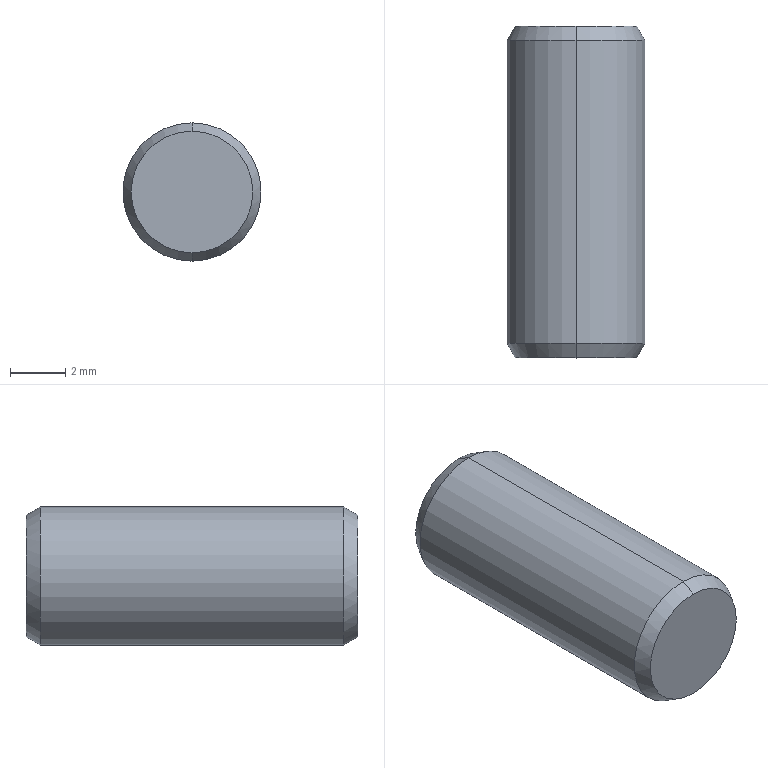Part | STEP file | 1 solid | 8 faces | box 5 x 12 x 5 mm | volume 233.269 mm3 | cone 4 | cylinder 2 | plane 2 | commonest cylinder face diameters 5 x2
STEP:
#1=CARTESIAN_POINT('',(0.,0.,0.));
#2=DIRECTION('',(0.,0.,1.));
#3=DIRECTION('',(1.,0.,0.));
#4=AXIS2_PLACEMENT_3D('',#1,#2,#3);
#5=CARTESIAN_POINT('',(0.,-12.,-2.2));
#6=VERTEX_POINT('',#5);
#7=CARTESIAN_POINT('',(0.,-12.,2.2));
#8=VERTEX_POINT('',#7);
#9=CARTESIAN_POINT('',(0.,-12.,0.));
#10=DIRECTION('',(0.,-1.,0.));
#11=DIRECTION('',(0.,0.,-1.));
#12=AXIS2_PLACEMENT_3D('',#9,#10,#11);
#13=CIRCLE('',#12,2.2);
#14=CARTESIAN_POINT('',(0.,-11.48,0.));
#15=DIRECTION('',(0.,1.,0.));
#16=DIRECTION('',(0.,0.,1.));
#17=AXIS2_PLACEMENT_3D('',#14,#15,#16);
#18=CONICAL_SURFACE('',#17,2.5,0.5236);
#19=CARTESIAN_POINT('',(3.142,-0.5196));
#20=DIRECTION('',(-1.,0.));
#21=VECTOR('',#20,1.);
#22=LINE('',#19,#21);
#23=(GEOMETRIC_REPRESENTATION_CONTEXT(2)PARAMETRIC_REPRESENTATION_CONTEXT()REPRESENTATION_CONTEXT('',''));
#24=DEFINITIONAL_REPRESENTATION('',(#22),#23);
#25=PCURVE('',#18,#24);
#26=CARTESIAN_POINT('',(-2.2,-12.,0.));
#27=DIRECTION('',(0.,1.,0.));
#28=DIRECTION('',(0.,0.,1.));
#29=AXIS2_PLACEMENT_3D('',#26,#27,#28);
#30=PLANE('',#29);
#31=CARTESIAN_POINT('',(-2.2,2.2));
#32=CARTESIAN_POINT('',(-2.2,6.011));
#33=CARTESIAN_POINT('',(1.1,4.105));
#34=CARTESIAN_POINT('',(4.4,2.2));
#35=CARTESIAN_POINT('',(1.1,0.2947));
#36=CARTESIAN_POINT('',(-2.2,-1.611));
#37=CARTESIAN_POINT('',(-2.2,2.2));
#38=(BOUNDED_CURVE()B_SPLINE_CURVE(2,(#31,#32,#33,#34,#35,#36,#37),.UNSPECIFIED.,.T.,.F.)B_SPLINE_CURVE_WITH_KNOTS((1,2,2,2,2,1),(-2.094,0.,2.094,4.189,6.283,8.378),.UNSPECIFIED.)CURVE()GEOMETRIC_REPRESENTATION_ITEM()RATIONAL_B_SPLINE_CURVE((1.,0.5,1.,0.5,1.,0.5,1.))REPRESENTATION_ITEM(''));
#39=(GEOMETRIC_REPRESENTATION_CONTEXT(2)PARAMETRIC_REPRESENTATION_CONTEXT()REPRESENTATION_CONTEXT('',''));
#40=DEFINITIONAL_REPRESENTATION('',(#38),#39);
#41=PCURVE('',#30,#40);
#42=SURFACE_CURVE('',#13,(#25,#41),.PCURVE_S1.);
#43=EDGE_CURVE('',#6,#8,#42,.T.);
#44=ORIENTED_EDGE('',*,*,#43,.F.);
#45=CARTESIAN_POINT('',(0.,-11.48,-2.5));
#46=VERTEX_POINT('',#45);
#47=CARTESIAN_POINT('',(0.,-11.48,-2.5));
#48=DIRECTION('',(0.,0.866,-0.5));
#49=VECTOR('',#48,1.);
#50=LINE('',#47,#49);
#51=CARTESIAN_POINT('',(3.142,0.));
#52=DIRECTION('',(0.,1.));
#53=VECTOR('',#52,1.);
#54=LINE('',#51,#53);
#55=(GEOMETRIC_REPRESENTATION_CONTEXT(2)PARAMETRIC_REPRESENTATION_CONTEXT()REPRESENTATION_CONTEXT('',''));
#56=DEFINITIONAL_REPRESENTATION('',(#54),#55);
#57=PCURVE('',#18,#56);
#58=CARTESIAN_POINT('',(0.,-11.48,0.));
#59=DIRECTION('',(0.,1.,0.));
#60=DIRECTION('',(0.,0.,1.));
#61=AXIS2_PLACEMENT_3D('',#58,#59,#60);
#62=CONICAL_SURFACE('',#61,2.5,0.5236);
#63=CARTESIAN_POINT('',(3.142,0.));
#64=DIRECTION('',(0.,1.));
#65=VECTOR('',#64,1.);
#66=LINE('',#63,#65);
#67=(GEOMETRIC_REPRESENTATION_CONTEXT(2)PARAMETRIC_REPRESENTATION_CONTEXT()REPRESENTATION_CONTEXT('',''));
#68=DEFINITIONAL_REPRESENTATION('',(#66),#67);
#69=PCURVE('',#62,#68);
#70=SURFACE_CURVE('',#50,(#57,#69),.PCURVE_S1.);
#71=EDGE_CURVE('',#6,#46,#70,.T.);
#72=ORIENTED_EDGE('',*,*,#71,.T.);
#73=CARTESIAN_POINT('',(0.,-11.48,2.5));
#74=VERTEX_POINT('',#73);
#75=CARTESIAN_POINT('',(0.,-11.48,0.));
#76=DIRECTION('',(0.,-1.,0.));
#77=DIRECTION('',(0.,0.,-1.));
#78=AXIS2_PLACEMENT_3D('',#75,#76,#77);
#79=CIRCLE('',#78,2.5);
#80=CARTESIAN_POINT('',(3.142,0.));
#81=DIRECTION('',(-1.,0.));
#82=VECTOR('',#81,1.);
#83=LINE('',#80,#82);
#84=(GEOMETRIC_REPRESENTATION_CONTEXT(2)PARAMETRIC_REPRESENTATION_CONTEXT()REPRESENTATION_CONTEXT('',''));
#85=DEFINITIONAL_REPRESENTATION('',(#83),#84);
#86=PCURVE('',#18,#85);
#87=CARTESIAN_POINT('',(0.,-12.,0.));
#88=DIRECTION('',(0.,-1.,0.));
#89=DIRECTION('',(0.,0.,-1.));
#90=AXIS2_PLACEMENT_3D('',#87,#88,#89);
#91=CYLINDRICAL_SURFACE('',#90,2.5);
#92=CARTESIAN_POINT('',(0.,-0.5196));
#93=DIRECTION('',(1.,0.));
#94=VECTOR('',#93,1.);
#95=LINE('',#92,#94);
#96=(GEOMETRIC_REPRESENTATION_CONTEXT(2)PARAMETRIC_REPRESENTATION_CONTEXT()REPRESENTATION_CONTEXT('',''));
#97=DEFINITIONAL_REPRESENTATION('',(#95),#96);
#98=PCURVE('',#91,#97);
#99=SURFACE_CURVE('',#79,(#86,#98),.PCURVE_S1.);
#100=EDGE_CURVE('',#46,#74,#99,.T.);
#101=ORIENTED_EDGE('',*,*,#100,.T.);
#102=CARTESIAN_POINT('',(0.,-11.48,2.5));
#103=DIRECTION('',(0.,0.866,0.5));
#104=VECTOR('',#103,1.);
#105=LINE('',#102,#104);
#106=CARTESIAN_POINT('',(0.,0.));
#107=DIRECTION('',(0.,1.));
#108=VECTOR('',#107,1.);
#109=LINE('',#106,#108);
#110=(GEOMETRIC_REPRESENTATION_CONTEXT(2)PARAMETRIC_REPRESENTATION_CONTEXT()REPRESENTATION_CONTEXT('',''));
#111=DEFINITIONAL_REPRESENTATION('',(#109),#110);
#112=PCURVE('',#18,#111);
#113=CARTESIAN_POINT('',(6.283,0.));
#114=DIRECTION('',(0.,1.));
#115=VECTOR('',#114,1.);
#116=LINE('',#113,#115);
#117=(GEOMETRIC_REPRESENTATION_CONTEXT(2)PARAMETRIC_REPRESENTATION_CONTEXT()REPRESENTATION_CONTEXT('',''));
#118=DEFINITIONAL_REPRESENTATION('',(#116),#117);
#119=PCURVE('',#62,#118);
#120=SURFACE_CURVE('',#105,(#112,#119),.PCURVE_S1.);
#121=EDGE_CURVE('',#8,#74,#120,.T.);
#122=ORIENTED_EDGE('',*,*,#121,.F.);
#123=EDGE_LOOP('',(#44,#72,#101,#122));
#124=FACE_BOUND('',#123,.T.);
#125=ADVANCED_FACE('',(#124),#18,.T.);
#126=CARTESIAN_POINT('',(0.,-0.5196,-2.5));
#127=VERTEX_POINT('',#126);
#128=CARTESIAN_POINT('',(0.,-0.5196,2.5));
#129=VERTEX_POINT('',#128);
#130=CARTESIAN_POINT('',(0.,-0.5196,0.));
#131=DIRECTION('',(0.,-1.,0.));
#132=DIRECTION('',(0.,0.,-1.));
#133=AXIS2_PLACEMENT_3D('',#130,#131,#132);
#134=CIRCLE('',#133,2.5);
#135=CARTESIAN_POINT('',(0.,-11.48));
#136=DIRECTION('',(1.,0.));
#137=VECTOR('',#136,1.);
#138=LINE('',#135,#137);
#139=(GEOMETRIC_REPRESENTATION_CONTEXT(2)PARAMETRIC_REPRESENTATION_CONTEXT()REPRESENTATION_CONTEXT('',''));
#140=DEFINITIONAL_REPRESENTATION('',(#138),#139);
#141=PCURVE('',#91,#140);
#142=CARTESIAN_POINT('',(0.,0.,0.));
#143=DIRECTION('',(0.,-1.,0.));
#144=DIRECTION('',(0.,0.,-1.));
#145=AXIS2_PLACEMENT_3D('',#142,#143,#144);
#146=CONICAL_SURFACE('',#145,2.2,0.5236);
#147=CARTESIAN_POINT('',(0.,0.5196));
#148=DIRECTION('',(1.,0.));
#149=VECTOR('',#148,1.);
#150=LINE('',#147,#149);
#151=(GEOMETRIC_REPRESENTATION_CONTEXT(2)PARAMETRIC_REPRESENTATION_CONTEXT()REPRESENTATION_CONTEXT('',''));
#152=DEFINITIONAL_REPRESENTATION('',(#150),#151);
#153=PCURVE('',#146,#152);
#154=SURFACE_CURVE('',#134,(#141,#153),.PCURVE_S1.);
#155=EDGE_CURVE('',#127,#129,#154,.T.);
#156=ORIENTED_EDGE('',*,*,#155,.T.);
#157=CARTESIAN_POINT('',(0.,-12.,2.5));
#158=DIRECTION('',(0.,-1.,0.));
#159=VECTOR('',#158,1.);
#160=LINE('',#157,#159);
#161=CARTESIAN_POINT('',(3.142,0.));
#162=DIRECTION('',(0.,1.));
#163=VECTOR('',#162,1.);
#164=LINE('',#161,#163);
#165=(GEOMETRIC_REPRESENTATION_CONTEXT(2)PARAMETRIC_REPRESENTATION_CONTEXT()REPRESENTATION_CONTEXT('',''));
#166=DEFINITIONAL_REPRESENTATION('',(#164),#165);
#167=PCURVE('',#91,#166);
#168=CARTESIAN_POINT('',(0.,-12.,0.));
#169=DIRECTION('',(0.,-1.,0.));
#170=DIRECTION('',(0.,0.,-1.));
#171=AXIS2_PLACEMENT_3D('',#168,#169,#170);
#172=CYLINDRICAL_SURFACE('',#171,2.5);
#173=CARTESIAN_POINT('',(3.142,0.));
#174=DIRECTION('',(0.,1.));
#175=VECTOR('',#174,1.);
#176=LINE('',#173,#175);
#177=(GEOMETRIC_REPRESENTATION_CONTEXT(2)PARAMETRIC_REPRESENTATION_CONTEXT()REPRESENTATION_CONTEXT('',''));
#178=DEFINITIONAL_REPRESENTATION('',(#176),#177);
#179=PCURVE('',#172,#178);
#180=SURFACE_CURVE('',#160,(#167,#179),.PCURVE_S1.);
#181=EDGE_CURVE('',#129,#74,#180,.T.);
#182=ORIENTED_EDGE('',*,*,#181,.T.);
#183=ORIENTED_EDGE('',*,*,#100,.F.);
#184=CARTESIAN_POINT('',(0.,-12.,-2.5));
#185=DIRECTION('',(0.,-1.,0.));
#186=VECTOR('',#185,1.);
#187=LINE('',#184,#186);
#188=CARTESIAN_POINT('',(0.,0.));
#189=DIRECTION('',(0.,1.));
#190=VECTOR('',#189,1.);
#191=LINE('',#188,#190);
#192=(GEOMETRIC_REPRESENTATION_CONTEXT(2)PARAMETRIC_REPRESENTATION_CONTEXT()REPRESENTATION_CONTEXT('',''));
#193=DEFINITIONAL_REPRESENTATION('',(#191),#192);
#194=PCURVE('',#91,#193);
#195=CARTESIAN_POINT('',(6.283,0.));
#196=DIRECTION('',(0.,1.));
#197=VECTOR('',#196,1.);
#198=LINE('',#195,#197);
#199=(GEOMETRIC_REPRESENTATION_CONTEXT(2)PARAMETRIC_REPRESENTATION_CONTEXT()REPRESENTATION_CONTEXT('',''));
#200=DEFINITIONAL_REPRESENTATION('',(#198),#199);
#201=PCURVE('',#172,#200);
#202=SURFACE_CURVE('',#187,(#194,#201),.PCURVE_S1.);
#203=EDGE_CURVE('',#127,#46,#202,.T.);
#204=ORIENTED_EDGE('',*,*,#203,.F.);
#205=EDGE_LOOP('',(#156,#182,#183,#204));
#206=FACE_BOUND('',#205,.T.);
#207=ADVANCED_FACE('',(#206),#91,.T.);
#208=CARTESIAN_POINT('',(0.,0.,-2.2));
#209=VERTEX_POINT('',#208);
#210=CARTESIAN_POINT('',(0.,0.,2.2));
#211=VERTEX_POINT('',#210);
#212=CARTESIAN_POINT('',(0.,0.,0.));
#213=DIRECTION('',(0.,-1.,0.));
#214=DIRECTION('',(0.,0.,-1.));
#215=AXIS2_PLACEMENT_3D('',#212,#213,#214);
#216=CIRCLE('',#215,2.2);
#217=CARTESIAN_POINT('',(0.,0.));
#218=DIRECTION('',(1.,0.));
#219=VECTOR('',#218,1.);
#220=LINE('',#217,#219);
#221=(GEOMETRIC_REPRESENTATION_CONTEXT(2)PARAMETRIC_REPRESENTATION_CONTEXT()REPRESENTATION_CONTEXT('',''));
#222=DEFINITIONAL_REPRESENTATION('',(#220),#221);
#223=PCURVE('',#146,#222);
#224=CARTESIAN_POINT('',(0.,0.,0.));
#225=DIRECTION('',(0.,-1.,0.));
#226=DIRECTION('',(0.,0.,-1.));
#227=AXIS2_PLACEMENT_3D('',#224,#225,#226);
#228=PLANE('',#227);
#229=CARTESIAN_POINT('',(0.,0.));
#230=DIRECTION('',(1.,0.));
#231=AXIS2_PLACEMENT_2D('',#229,#230);
#232=CIRCLE('',#231,2.2);
#233=(GEOMETRIC_REPRESENTATION_CONTEXT(2)PARAMETRIC_REPRESENTATION_CONTEXT()REPRESENTATION_CONTEXT('',''));
#234=DEFINITIONAL_REPRESENTATION('',(#232),#233);
#235=PCURVE('',#228,#234);
#236=SURFACE_CURVE('',#216,(#223,#235),.PCURVE_S1.);
#237=EDGE_CURVE('',#209,#211,#236,.T.);
#238=ORIENTED_EDGE('',*,*,#237,.T.);
#239=CARTESIAN_POINT('',(0.,0.,2.2));
#240=DIRECTION('',(0.,-0.866,0.5));
#241=VECTOR('',#240,1.);
#242=LINE('',#239,#241);
#243=CARTESIAN_POINT('',(3.142,0.));
#244=DIRECTION('',(0.,1.));
#245=VECTOR('',#244,1.);
#246=LINE('',#243,#245);
#247=(GEOMETRIC_REPRESENTATION_CONTEXT(2)PARAMETRIC_REPRESENTATION_CONTEXT()REPRESENTATION_CONTEXT('',''));
#248=DEFINITIONAL_REPRESENTATION('',(#246),#247);
#249=PCURVE('',#146,#248);
#250=CARTESIAN_POINT('',(0.,0.,0.));
#251=DIRECTION('',(0.,-1.,0.));
#252=DIRECTION('',(0.,0.,-1.));
#253=AXIS2_PLACEMENT_3D('',#250,#251,#252);
#254=CONICAL_SURFACE('',#253,2.2,0.5236);
#255=CARTESIAN_POINT('',(3.142,0.));
#256=DIRECTION('',(0.,1.));
#257=VECTOR('',#256,1.);
#258=LINE('',#255,#257);
#259=(GEOMETRIC_REPRESENTATION_CONTEXT(2)PARAMETRIC_REPRESENTATION_CONTEXT()REPRESENTATION_CONTEXT('',''));
#260=DEFINITIONAL_REPRESENTATION('',(#258),#259);
#261=PCURVE('',#254,#260);
#262=SURFACE_CURVE('',#242,(#249,#261),.PCURVE_S1.);
#263=EDGE_CURVE('',#211,#129,#262,.T.);
#264=ORIENTED_EDGE('',*,*,#263,.T.);
#265=ORIENTED_EDGE('',*,*,#155,.F.);
#266=CARTESIAN_POINT('',(0.,0.,-2.2));
#267=DIRECTION('',(0.,-0.866,-0.5));
#268=VECTOR('',#267,1.);
#269=LINE('',#266,#268);
#270=CARTESIAN_POINT('',(0.,0.));
#271=DIRECTION('',(0.,1.));
#272=VECTOR('',#271,1.);
#273=LINE('',#270,#272);
#274=(GEOMETRIC_REPRESENTATION_CONTEXT(2)PARAMETRIC_REPRESENTATION_CONTEXT()REPRESENTATION_CONTEXT('',''));
#275=DEFINITIONAL_REPRESENTATION('',(#273),#274);
#276=PCURVE('',#146,#275);
#277=CARTESIAN_POINT('',(6.283,0.));
#278=DIRECTION('',(0.,1.));
#279=VECTOR('',#278,1.);
#280=LINE('',#277,#279);
#281=(GEOMETRIC_REPRESENTATION_CONTEXT(2)PARAMETRIC_REPRESENTATION_CONTEXT()REPRESENTATION_CONTEXT('',''));
#282=DEFINITIONAL_REPRESENTATION('',(#280),#281);
#283=PCURVE('',#254,#282);
#284=SURFACE_CURVE('',#269,(#276,#283),.PCURVE_S1.);
#285=EDGE_CURVE('',#209,#127,#284,.T.);
#286=ORIENTED_EDGE('',*,*,#285,.F.);
#287=EDGE_LOOP('',(#238,#264,#265,#286));
#288=FACE_BOUND('',#287,.T.);
#289=ADVANCED_FACE('',(#288),#146,.T.);
#290=ORIENTED_EDGE('',*,*,#263,.F.);
#291=CARTESIAN_POINT('',(0.,0.,0.));
#292=DIRECTION('',(0.,-1.,0.));
#293=DIRECTION('',(0.,0.,-1.));
#294=AXIS2_PLACEMENT_3D('',#291,#292,#293);
#295=CIRCLE('',#294,2.2);
#296=CARTESIAN_POINT('',(0.,0.));
#297=DIRECTION('',(1.,0.));
#298=VECTOR('',#297,1.);
#299=LINE('',#296,#298);
#300=(GEOMETRIC_REPRESENTATION_CONTEXT(2)PARAMETRIC_REPRESENTATION_CONTEXT()REPRESENTATION_CONTEXT('',''));
#301=DEFINITIONAL_REPRESENTATION('',(#299),#300);
#302=PCURVE('',#254,#301);
#303=CARTESIAN_POINT('',(0.,0.));
#304=DIRECTION('',(1.,0.));
#305=AXIS2_PLACEMENT_2D('',#303,#304);
#306=CIRCLE('',#305,2.2);
#307=(GEOMETRIC_REPRESENTATION_CONTEXT(2)PARAMETRIC_REPRESENTATION_CONTEXT()REPRESENTATION_CONTEXT('',''));
#308=DEFINITIONAL_REPRESENTATION('',(#306),#307);
#309=PCURVE('',#228,#308);
#310=SURFACE_CURVE('',#295,(#302,#309),.PCURVE_S1.);
#311=EDGE_CURVE('',#211,#209,#310,.T.);
#312=ORIENTED_EDGE('',*,*,#311,.T.);
#313=ORIENTED_EDGE('',*,*,#285,.T.);
#314=CARTESIAN_POINT('',(0.,-0.5196,0.));
#315=DIRECTION('',(0.,-1.,0.));
#316=DIRECTION('',(0.,0.,-1.));
#317=AXIS2_PLACEMENT_3D('',#314,#315,#316);
#318=CIRCLE('',#317,2.5);
#319=CARTESIAN_POINT('',(0.,0.5196));
#320=DIRECTION('',(1.,0.));
#321=VECTOR('',#320,1.);
#322=LINE('',#319,#321);
#323=(GEOMETRIC_REPRESENTATION_CONTEXT(2)PARAMETRIC_REPRESENTATION_CONTEXT()REPRESENTATION_CONTEXT('',''));
#324=DEFINITIONAL_REPRESENTATION('',(#322),#323);
#325=PCURVE('',#254,#324);
#326=CARTESIAN_POINT('',(0.,-11.48));
#327=DIRECTION('',(1.,0.));
#328=VECTOR('',#327,1.);
#329=LINE('',#326,#328);
#330=(GEOMETRIC_REPRESENTATION_CONTEXT(2)PARAMETRIC_REPRESENTATION_CONTEXT()REPRESENTATION_CONTEXT('',''));
#331=DEFINITIONAL_REPRESENTATION('',(#329),#330);
#332=PCURVE('',#172,#331);
#333=SURFACE_CURVE('',#318,(#325,#332),.PCURVE_S1.);
#334=EDGE_CURVE('',#129,#127,#333,.T.);
#335=ORIENTED_EDGE('',*,*,#334,.F.);
#336=EDGE_LOOP('',(#290,#312,#313,#335));
#337=FACE_BOUND('',#336,.T.);
#338=ADVANCED_FACE('',(#337),#254,.T.);
#339=ORIENTED_EDGE('',*,*,#181,.F.);
#340=ORIENTED_EDGE('',*,*,#334,.T.);
#341=ORIENTED_EDGE('',*,*,#203,.T.);
#342=CARTESIAN_POINT('',(0.,-11.48,0.));
#343=DIRECTION('',(0.,-1.,0.));
#344=DIRECTION('',(0.,0.,-1.));
#345=AXIS2_PLACEMENT_3D('',#342,#343,#344);
#346=CIRCLE('',#345,2.5);
#347=CARTESIAN_POINT('',(0.,-0.5196));
#348=DIRECTION('',(1.,0.));
#349=VECTOR('',#348,1.);
#350=LINE('',#347,#349);
#351=(GEOMETRIC_REPRESENTATION_CONTEXT(2)PARAMETRIC_REPRESENTATION_CONTEXT()REPRESENTATION_CONTEXT('',''));
#352=DEFINITIONAL_REPRESENTATION('',(#350),#351);
#353=PCURVE('',#172,#352);
#354=CARTESIAN_POINT('',(9.425,0.));
#355=DIRECTION('',(-1.,0.));
#356=VECTOR('',#355,1.);
#357=LINE('',#354,#356);
#358=(GEOMETRIC_REPRESENTATION_CONTEXT(2)PARAMETRIC_REPRESENTATION_CONTEXT()REPRESENTATION_CONTEXT('',''));
#359=DEFINITIONAL_REPRESENTATION('',(#357),#358);
#360=PCURVE('',#62,#359);
#361=SURFACE_CURVE('',#346,(#353,#360),.PCURVE_S1.);
#362=EDGE_CURVE('',#74,#46,#361,.T.);
#363=ORIENTED_EDGE('',*,*,#362,.F.);
#364=EDGE_LOOP('',(#339,#340,#341,#363));
#365=FACE_BOUND('',#364,.T.);
#366=ADVANCED_FACE('',(#365),#172,.T.);
#367=ORIENTED_EDGE('',*,*,#71,.F.);
#368=CARTESIAN_POINT('',(0.,-12.,0.));
#369=DIRECTION('',(0.,-1.,0.));
#370=DIRECTION('',(0.,0.,-1.));
#371=AXIS2_PLACEMENT_3D('',#368,#369,#370);
#372=CIRCLE('',#371,2.2);
#373=CARTESIAN_POINT('',(9.425,-0.5196));
#374=DIRECTION('',(-1.,0.));
#375=VECTOR('',#374,1.);
#376=LINE('',#373,#375);
#377=(GEOMETRIC_REPRESENTATION_CONTEXT(2)PARAMETRIC_REPRESENTATION_CONTEXT()REPRESENTATION_CONTEXT('',''));
#378=DEFINITIONAL_REPRESENTATION('',(#376),#377);
#379=PCURVE('',#62,#378);
#380=CARTESIAN_POINT('',(-2.2,2.2));
#381=CARTESIAN_POINT('',(-2.2,6.011));
#382=CARTESIAN_POINT('',(1.1,4.105));
#383=CARTESIAN_POINT('',(4.4,2.2));
#384=CARTESIAN_POINT('',(1.1,0.2947));
#385=CARTESIAN_POINT('',(-2.2,-1.611));
#386=CARTESIAN_POINT('',(-2.2,2.2));
#387=(BOUNDED_CURVE()B_SPLINE_CURVE(2,(#380,#381,#382,#383,#384,#385,#386),.UNSPECIFIED.,.T.,.F.)B_SPLINE_CURVE_WITH_KNOTS((1,2,2,2,2,1),(-2.094,0.,2.094,4.189,6.283,8.378),.UNSPECIFIED.)CURVE()GEOMETRIC_REPRESENTATION_ITEM()RATIONAL_B_SPLINE_CURVE((1.,0.5,1.,0.5,1.,0.5,1.))REPRESENTATION_ITEM(''));
#388=(GEOMETRIC_REPRESENTATION_CONTEXT(2)PARAMETRIC_REPRESENTATION_CONTEXT()REPRESENTATION_CONTEXT('',''));
#389=DEFINITIONAL_REPRESENTATION('',(#387),#388);
#390=PCURVE('',#30,#389);
#391=SURFACE_CURVE('',#372,(#379,#390),.PCURVE_S1.);
#392=EDGE_CURVE('',#8,#6,#391,.T.);
#393=ORIENTED_EDGE('',*,*,#392,.F.);
#394=ORIENTED_EDGE('',*,*,#121,.T.);
#395=ORIENTED_EDGE('',*,*,#362,.T.);
#396=EDGE_LOOP('',(#367,#393,#394,#395));
#397=FACE_BOUND('',#396,.T.);
#398=ADVANCED_FACE('',(#397),#62,.T.);
#399=ORIENTED_EDGE('',*,*,#392,.T.);
#400=ORIENTED_EDGE('',*,*,#43,.T.);
#401=EDGE_LOOP('',(#399,#400));
#402=FACE_BOUND('',#401,.T.);
#403=ADVANCED_FACE('',(#402),#30,.F.);
#404=ORIENTED_EDGE('',*,*,#237,.F.);
#405=ORIENTED_EDGE('',*,*,#311,.F.);
#406=EDGE_LOOP('',(#404,#405));
#407=FACE_BOUND('',#406,.T.);
#408=ADVANCED_FACE('',(#407),#228,.F.);
#409=CLOSED_SHELL('',(#125,#207,#289,#338,#366,#398,#403,#408));
#410=MANIFOLD_SOLID_BREP('',#409);
#411=(LENGTH_UNIT()NAMED_UNIT(*)SI_UNIT(.MILLI.,.METRE.));
#412=UNCERTAINTY_MEASURE_WITH_UNIT(LENGTH_MEASURE(0.0000001),#411,'','');
#413=(NAMED_UNIT(*)PLANE_ANGLE_UNIT()SI_UNIT($,.RADIAN.));
#414=(NAMED_UNIT(*)SI_UNIT($,.STERADIAN.)SOLID_ANGLE_UNIT());
#415=(GEOMETRIC_REPRESENTATION_CONTEXT(3)GLOBAL_UNCERTAINTY_ASSIGNED_CONTEXT((#412))GLOBAL_UNIT_ASSIGNED_CONTEXT((#411,#413,#414))REPRESENTATION_CONTEXT('',''));
#416=ADVANCED_BREP_SHAPE_REPRESENTATION('',(#4,#410),#415);